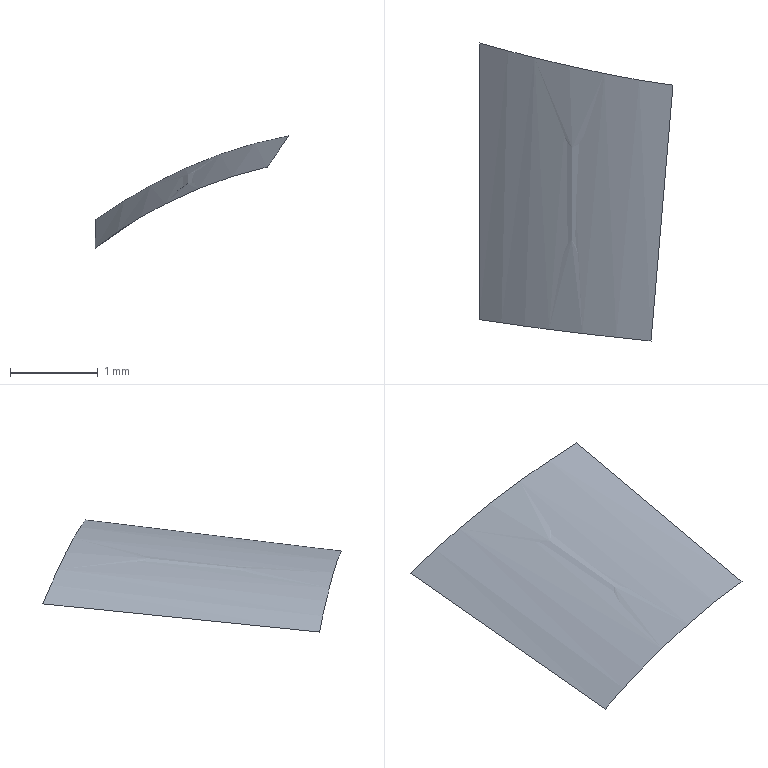Part | NX | features solid 2 | 1 solid | 2 faces | box 2.2 x 3.401 x 1.283 mm | volume 0.002967 mm3 | spline 2